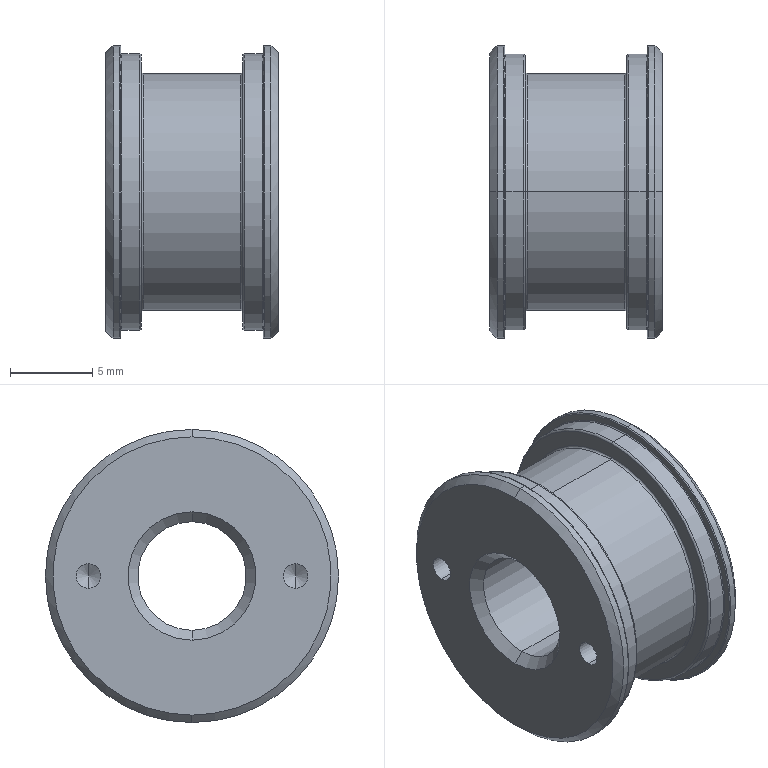Part | STEP file | 2026.6.15-Main Assembly图.sldasm-Part-167 | 1 solid | 68 faces | box 10.5 x 17.82 x 17.82 mm | volume 1584 mm3 | torus 24 | cylinder 22 | cone 14 | plane 8 | commonest cylinder face diameters 1.5 x4 7.5 x4 16.8 x4 17.82 x4 6.6 x2 8.85 x2